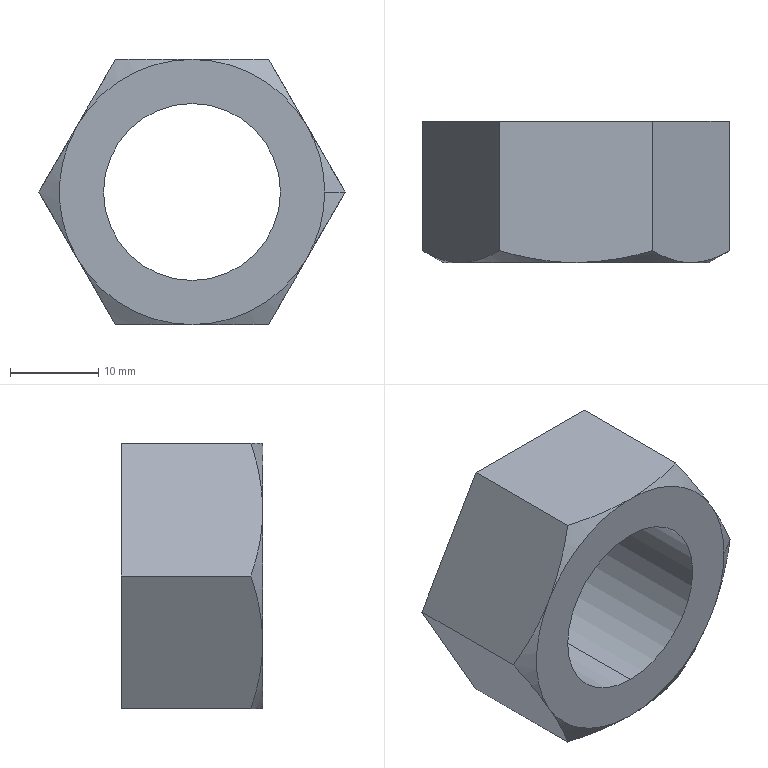Part | STEP file | SCHI20-Part-1 | 1 solid | 17 faces | box 34.641 x 16 x 30 mm | volume 7415 mm3 | plane 8 | cone 7 | cylinder 2 | commonest cylinder face diameters 20 x2